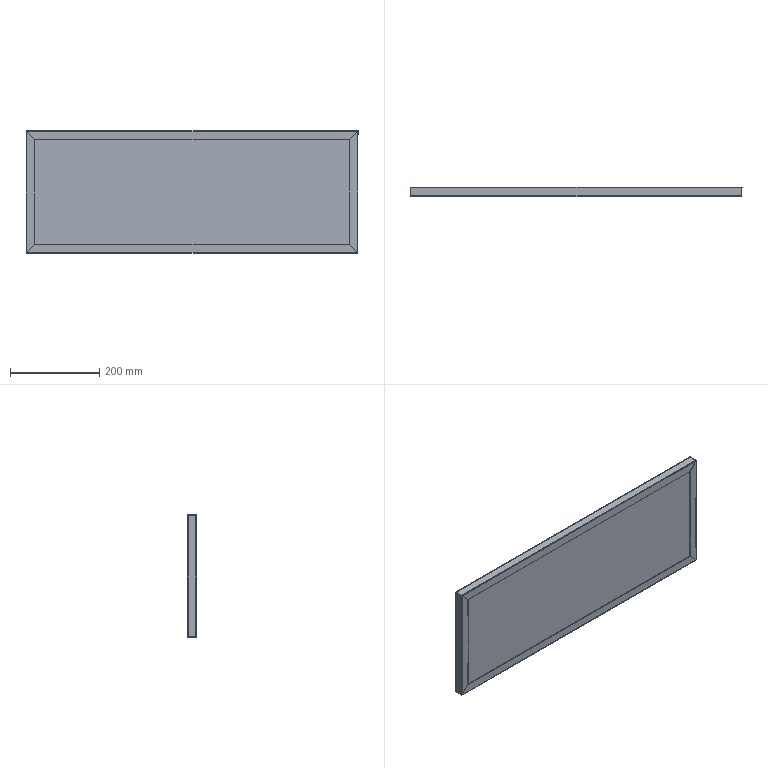Part | SolidWorks | features CornerFeat 1, FlatPattern 1, FlattenBends 1, ProcessBends 1, SheetMetal 1, SplitBody 1 | 1 solid | 86 faces | box 745 x 20 x 273.8 mm | volume 278470 mm3 | plane 54 | spline 16 | cylinder 16 | commonest cylinder face diameters 0.4 x8 2.4 x8